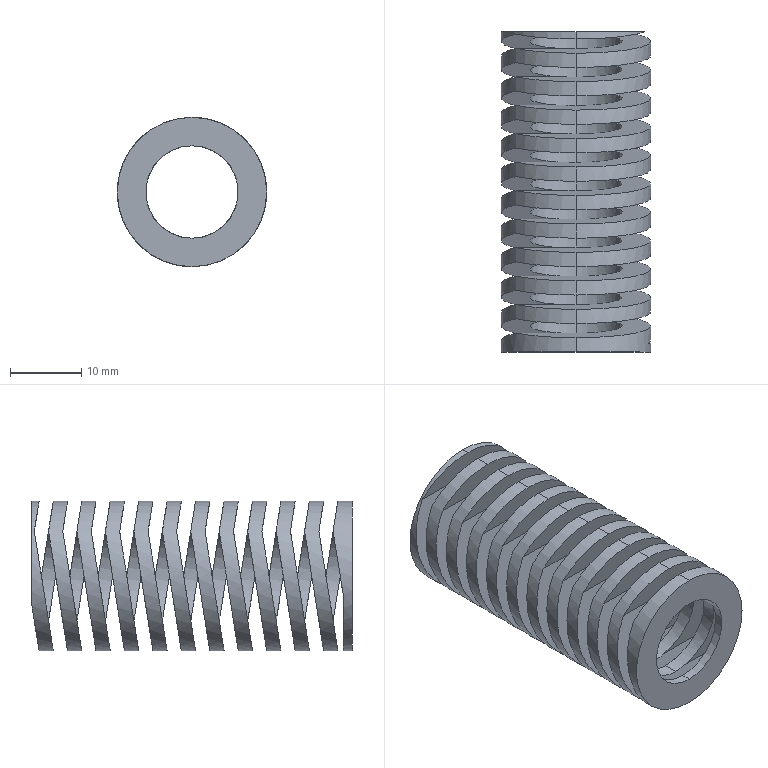Part | STEP file | 001-009-YSWC-D21-L45 | 1 solid | 97 faces | box 21 x 45 x 21 mm | volume 4940 mm3 | plane 49 | cylinder 48 | commonest cylinder face diameters 13 x24 21 x24